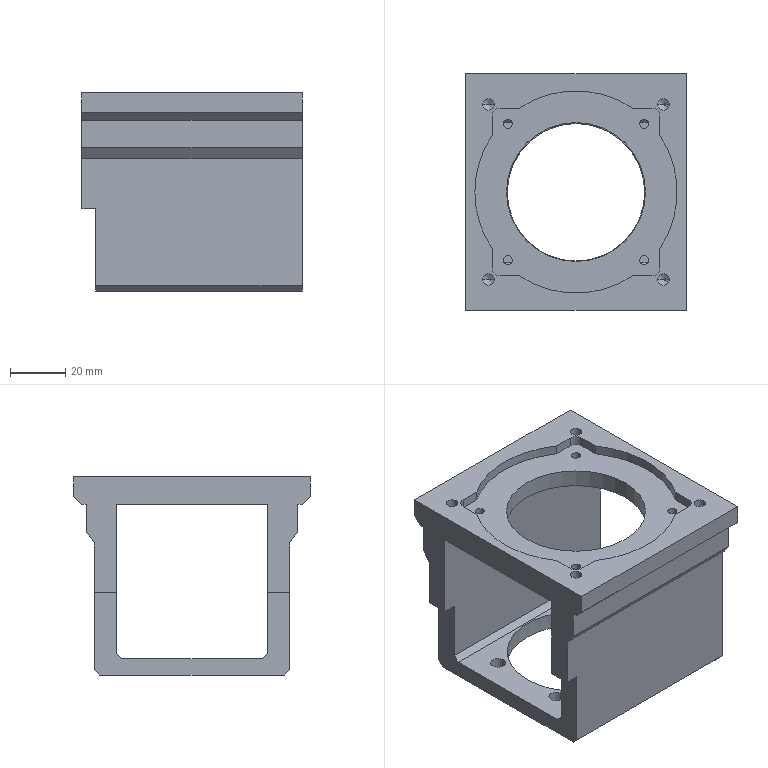Part | NX | features BREP 1 | 1 solid | 91 faces | box 80 x 86 x 72 mm | volume 133305 mm3 | cylinder 43 | plane 40 | cone 8 | commonest cylinder face diameters 3.3 x8 4.2 x8 5.5 x8 8 x6 73.5 x5 6 x4